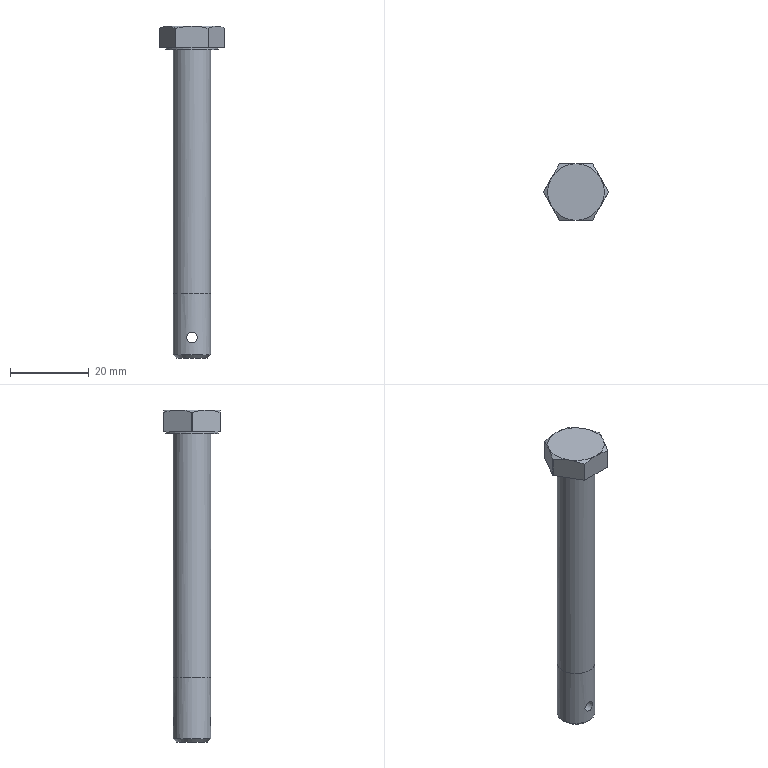Part | NX | features solid 2 | 1 solid | 27 faces | box 16.51 x 14.351 x 84.153 mm | volume 6554 mm3 | cylinder 10 | plane 10 | cone 7 | commonest cylinder face diameters 16.51 x6 9.525 x2 2.692 x1 13.284 x1
STEP:
#1=CARTESIAN_POINT('',(0.,-4.763,-80.34));
#2=VERTEX_POINT('',#1);
#3=CARTESIAN_POINT('',(1.056,-4.667,-80.048));
#4=CARTESIAN_POINT('',(-0.0001384,-4.81,-80.486));
#5=CARTESIAN_POINT('',(-1.055,-4.667,-80.048));
#6=CARTESIAN_POINT('',(-1.492,-4.519,-78.996));
#7=CARTESIAN_POINT('',(-1.055,-4.667,-77.939));
#8=CARTESIAN_POINT('',(-0.0007508,-4.81,-77.502));
#9=CARTESIAN_POINT('',(1.054,-4.668,-77.938));
#10=CARTESIAN_POINT('',(1.492,-4.519,-78.994));
#11=CARTESIAN_POINT('',(1.056,-4.667,-80.048));
#12=CARTESIAN_POINT('',(-0.0001384,-4.81,-80.486));
#13=CARTESIAN_POINT('',(-1.055,-4.667,-80.048));
#14=B_SPLINE_CURVE_WITH_KNOTS('',3,(#3,#4,#5,#6,#7,#8,#9,#10,#11,#12,#13),.UNSPECIFIED.,.T.,.F.,(1,1,1,1,1,1,1,1,1,1,1,1,1,1,1),(-0.003172,-0.002115,-0.001057,0.,0.001057,0.002115,0.003172,0.00423,0.005287,0.006345,0.007402,0.00846,0.009517,0.01057,0.01163),.UNSPECIFIED.);
#15=EDGE_CURVE('',#2,#2,#14,.T.);
#16=ORIENTED_EDGE('',*,*,#15,.T.);
#17=EDGE_LOOP('',(#16));
#18=FACE_BOUND('',#17,.T.);
#19=CARTESIAN_POINT('',(-4.763,0.,-67.882));
#20=VERTEX_POINT('',#19);
#21=CARTESIAN_POINT('',(-3.732,3.732,-67.882));
#22=CARTESIAN_POINT('',(-5.278,0.,-67.882));
#23=CARTESIAN_POINT('',(-3.732,-3.732,-67.882));
#24=CARTESIAN_POINT('',(0.,-5.278,-67.882));
#25=CARTESIAN_POINT('',(3.732,-3.732,-67.882));
#26=CARTESIAN_POINT('',(5.278,0.,-67.882));
#27=CARTESIAN_POINT('',(3.732,3.732,-67.882));
#28=CARTESIAN_POINT('',(0.,5.278,-67.882));
#29=CARTESIAN_POINT('',(-3.732,3.732,-67.882));
#30=CARTESIAN_POINT('',(-5.278,0.,-67.882));
#31=CARTESIAN_POINT('',(-3.732,-3.732,-67.882));
#32=B_SPLINE_CURVE_WITH_KNOTS('',3,(#21,#22,#23,#24,#25,#26,#27,#28,#29,#30,#31),.UNSPECIFIED.,.T.,.F.,(1,1,1,1,1,1,1,1,1,1,1,1,1,1,1),(-0.375,-0.25,-0.125,0.,0.125,0.25,0.375,0.5,0.625,0.75,0.875,1.,1.125,1.25,1.375),.UNSPECIFIED.);
#33=EDGE_CURVE('',#20,#20,#32,.T.);
#34=ORIENTED_EDGE('',*,*,#33,.F.);
#35=EDGE_LOOP('',(#34));
#36=FACE_BOUND('',#35,.T.);
#37=CARTESIAN_POINT('',(-4.763,0.,-83.366));
#38=VERTEX_POINT('',#37);
#39=CARTESIAN_POINT('',(0.,0.,-83.366));
#40=DIRECTION('',(0.,0.,-1.));
#41=DIRECTION('',(-1.,0.,0.));
#42=AXIS2_PLACEMENT_3D('',#39,#40,#41);
#43=CIRCLE('',#42,4.763);
#44=EDGE_CURVE('',#38,#38,#43,.T.);
#45=ORIENTED_EDGE('',*,*,#44,.F.);
#46=EDGE_LOOP('',(#45));
#47=FACE_BOUND('',#46,.T.);
#48=CARTESIAN_POINT('',(0.,4.763,-80.34));
#49=VERTEX_POINT('',#48);
#50=CARTESIAN_POINT('',(-1.056,4.667,-80.048));
#51=CARTESIAN_POINT('',(0.0001384,4.81,-80.486));
#52=CARTESIAN_POINT('',(1.055,4.667,-80.048));
#53=CARTESIAN_POINT('',(1.492,4.519,-78.996));
#54=CARTESIAN_POINT('',(1.055,4.667,-77.939));
#55=CARTESIAN_POINT('',(0.0007508,4.81,-77.502));
#56=CARTESIAN_POINT('',(-1.054,4.668,-77.938));
#57=CARTESIAN_POINT('',(-1.492,4.519,-78.994));
#58=CARTESIAN_POINT('',(-1.056,4.667,-80.048));
#59=CARTESIAN_POINT('',(0.0001384,4.81,-80.486));
#60=CARTESIAN_POINT('',(1.055,4.667,-80.048));
#61=B_SPLINE_CURVE_WITH_KNOTS('',3,(#50,#51,#52,#53,#54,#55,#56,#57,#58,#59,#60),.UNSPECIFIED.,.T.,.F.,(1,1,1,1,1,1,1,1,1,1,1,1,1,1,1),(-0.003172,-0.002115,-0.001057,0.,0.001057,0.002115,0.003172,0.00423,0.005287,0.006345,0.007402,0.00846,0.009517,0.01057,0.01163),.UNSPECIFIED.);
#62=EDGE_CURVE('',#49,#49,#61,.T.);
#63=ORIENTED_EDGE('',*,*,#62,.T.);
#64=EDGE_LOOP('',(#63));
#65=FACE_BOUND('',#64,.T.);
#66=CARTESIAN_POINT('',(0.,0.,0.));
#67=DIRECTION('',(0.,0.,-1.));
#68=DIRECTION('',(-1.,0.,0.));
#69=AXIS2_PLACEMENT_3D('',#66,#67,#68);
#70=CYLINDRICAL_SURFACE('',#69,4.763);
#71=ADVANCED_FACE('',(#18,#36,#47,#65),#70,.T.);
#72=CARTESIAN_POINT('',(-4.763,0.,-5.969));
#73=VERTEX_POINT('',#72);
#74=CARTESIAN_POINT('',(0.,0.,-5.969));
#75=DIRECTION('',(0.,0.,-1.));
#76=DIRECTION('',(-1.,0.,0.));
#77=AXIS2_PLACEMENT_3D('',#74,#75,#76);
#78=CIRCLE('',#77,4.763);
#79=EDGE_CURVE('',#73,#73,#78,.T.);
#80=ORIENTED_EDGE('',*,*,#79,.T.);
#81=EDGE_LOOP('',(#80));
#82=FACE_BOUND('',#81,.T.);
#83=ORIENTED_EDGE('',*,*,#33,.T.);
#84=EDGE_LOOP('',(#83));
#85=FACE_BOUND('',#84,.T.);
#86=CARTESIAN_POINT('',(0.,0.,0.));
#87=DIRECTION('',(0.,0.,-1.));
#88=DIRECTION('',(-1.,0.,0.));
#89=AXIS2_PLACEMENT_3D('',#86,#87,#88);
#90=CYLINDRICAL_SURFACE('',#89,4.763);
#91=ADVANCED_FACE('',(#82,#85),#90,.T.);
#92=CARTESIAN_POINT('',(4.081,7.176,-5.563));
#93=VERTEX_POINT('',#92);
#94=CARTESIAN_POINT('',(4.174,7.122,-5.563));
#95=VERTEX_POINT('',#94);
#96=CARTESIAN_POINT('',(0.,0.,-5.563));
#97=DIRECTION('',(0.,0.,-1.));
#98=DIRECTION('',(-1.,0.,0.));
#99=AXIS2_PLACEMENT_3D('',#96,#97,#98);
#100=CIRCLE('',#99,8.255);
#101=EDGE_CURVE('',#93,#95,#100,.T.);
#102=ORIENTED_EDGE('',*,*,#101,.F.);
#103=CARTESIAN_POINT('',(4.081,7.176,-0.6232));
#104=VERTEX_POINT('',#103);
#105=CARTESIAN_POINT('',(4.081,7.176,0.));
#106=DIRECTION('',(0.,0.,-1.));
#107=VECTOR('',#106,1000.);
#108=LINE('',#105,#107);
#109=EDGE_CURVE('',#93,#104,#108,.F.);
#110=ORIENTED_EDGE('',*,*,#109,.T.);
#111=CARTESIAN_POINT('',(4.174,7.122,-0.6232));
#112=VERTEX_POINT('',#111);
#113=CARTESIAN_POINT('',(0.,0.,-0.6232));
#114=DIRECTION('',(0.,0.,-1.));
#115=DIRECTION('',(-1.,0.,0.));
#116=AXIS2_PLACEMENT_3D('',#113,#114,#115);
#117=CIRCLE('',#116,8.255);
#118=EDGE_CURVE('',#104,#112,#117,.T.);
#119=ORIENTED_EDGE('',*,*,#118,.T.);
#120=CARTESIAN_POINT('',(4.174,7.122,0.));
#121=DIRECTION('',(0.,0.,-1.));
#122=VECTOR('',#121,1000.);
#123=LINE('',#120,#122);
#124=EDGE_CURVE('',#112,#95,#123,.T.);
#125=ORIENTED_EDGE('',*,*,#124,.T.);
#126=EDGE_LOOP('',(#102,#110,#119,#125));
#127=FACE_BOUND('',#126,.T.);
#128=CARTESIAN_POINT('',(0.,0.,0.));
#129=DIRECTION('',(0.,0.,-1.));
#130=DIRECTION('',(-1.,0.,0.));
#131=AXIS2_PLACEMENT_3D('',#128,#129,#130);
#132=CYLINDRICAL_SURFACE('',#131,8.255);
#133=ADVANCED_FACE('',(#127),#132,.T.);
#134=CARTESIAN_POINT('',(-4.174,7.122,-0.6232));
#135=VERTEX_POINT('',#134);
#136=CARTESIAN_POINT('',(-4.081,7.176,-0.6232));
#137=VERTEX_POINT('',#136);
#138=CARTESIAN_POINT('',(0.,0.,-0.6232));
#139=DIRECTION('',(0.,0.,-1.));
#140=DIRECTION('',(-1.,0.,0.));
#141=AXIS2_PLACEMENT_3D('',#138,#139,#140);
#142=CIRCLE('',#141,8.255);
#143=EDGE_CURVE('',#135,#137,#142,.T.);
#144=ORIENTED_EDGE('',*,*,#143,.T.);
#145=CARTESIAN_POINT('',(-4.081,7.176,-5.563));
#146=VERTEX_POINT('',#145);
#147=CARTESIAN_POINT('',(-4.081,7.176,0.));
#148=DIRECTION('',(0.,0.,-1.));
#149=VECTOR('',#148,1000.);
#150=LINE('',#147,#149);
#151=EDGE_CURVE('',#137,#146,#150,.T.);
#152=ORIENTED_EDGE('',*,*,#151,.T.);
#153=CARTESIAN_POINT('',(-4.174,7.122,-5.563));
#154=VERTEX_POINT('',#153);
#155=CARTESIAN_POINT('',(0.,0.,-5.563));
#156=DIRECTION('',(0.,0.,-1.));
#157=DIRECTION('',(-1.,0.,0.));
#158=AXIS2_PLACEMENT_3D('',#155,#156,#157);
#159=CIRCLE('',#158,8.255);
#160=EDGE_CURVE('',#154,#146,#159,.T.);
#161=ORIENTED_EDGE('',*,*,#160,.F.);
#162=CARTESIAN_POINT('',(-4.174,7.122,0.));
#163=DIRECTION('',(0.,0.,-1.));
#164=VECTOR('',#163,1000.);
#165=LINE('',#162,#164);
#166=EDGE_CURVE('',#154,#135,#165,.F.);
#167=ORIENTED_EDGE('',*,*,#166,.T.);
#168=EDGE_LOOP('',(#144,#152,#161,#167));
#169=FACE_BOUND('',#168,.T.);
#170=CARTESIAN_POINT('',(0.,0.,0.));
#171=DIRECTION('',(0.,0.,-1.));
#172=DIRECTION('',(-1.,0.,0.));
#173=AXIS2_PLACEMENT_3D('',#170,#171,#172);
#174=CYLINDRICAL_SURFACE('',#173,8.255);
#175=ADVANCED_FACE('',(#169),#174,.T.);
#176=CARTESIAN_POINT('',(-8.255,-0.05322,-0.6232));
#177=VERTEX_POINT('',#176);
#178=CARTESIAN_POINT('',(-8.255,0.05322,-0.6232));
#179=VERTEX_POINT('',#178);
#180=CARTESIAN_POINT('',(0.,0.,-0.6232));
#181=DIRECTION('',(0.,0.,-1.));
#182=DIRECTION('',(-1.,0.,0.));
#183=AXIS2_PLACEMENT_3D('',#180,#181,#182);
#184=CIRCLE('',#183,8.255);
#185=EDGE_CURVE('',#177,#179,#184,.T.);
#186=ORIENTED_EDGE('',*,*,#185,.T.);
#187=CARTESIAN_POINT('',(-8.255,0.05322,-5.563));
#188=VERTEX_POINT('',#187);
#189=CARTESIAN_POINT('',(-8.255,0.05322,0.));
#190=DIRECTION('',(0.,0.,-1.));
#191=VECTOR('',#190,1000.);
#192=LINE('',#189,#191);
#193=EDGE_CURVE('',#179,#188,#192,.T.);
#194=ORIENTED_EDGE('',*,*,#193,.T.);
#195=CARTESIAN_POINT('',(-8.255,-0.05322,-5.563));
#196=VERTEX_POINT('',#195);
#197=CARTESIAN_POINT('',(0.,0.,-5.563));
#198=DIRECTION('',(0.,0.,-1.));
#199=DIRECTION('',(-1.,0.,0.));
#200=AXIS2_PLACEMENT_3D('',#197,#198,#199);
#201=CIRCLE('',#200,8.255);
#202=EDGE_CURVE('',#196,#188,#201,.T.);
#203=ORIENTED_EDGE('',*,*,#202,.F.);
#204=CARTESIAN_POINT('',(-8.255,-0.05322,0.));
#205=DIRECTION('',(0.,0.,-1.));
#206=VECTOR('',#205,1000.);
#207=LINE('',#204,#206);
#208=EDGE_CURVE('',#196,#177,#207,.F.);
#209=ORIENTED_EDGE('',*,*,#208,.T.);
#210=EDGE_LOOP('',(#186,#194,#203,#209));
#211=FACE_BOUND('',#210,.T.);
#212=CARTESIAN_POINT('',(0.,0.,0.));
#213=DIRECTION('',(0.,0.,-1.));
#214=DIRECTION('',(-1.,0.,0.));
#215=AXIS2_PLACEMENT_3D('',#212,#213,#214);
#216=CYLINDRICAL_SURFACE('',#215,8.255);
#217=ADVANCED_FACE('',(#211),#216,.T.);
#218=CARTESIAN_POINT('',(-4.081,-7.176,-0.6232));
#219=VERTEX_POINT('',#218);
#220=CARTESIAN_POINT('',(-4.174,-7.122,-0.6232));
#221=VERTEX_POINT('',#220);
#222=CARTESIAN_POINT('',(0.,0.,-0.6232));
#223=DIRECTION('',(0.,0.,-1.));
#224=DIRECTION('',(-1.,0.,0.));
#225=AXIS2_PLACEMENT_3D('',#222,#223,#224);
#226=CIRCLE('',#225,8.255);
#227=EDGE_CURVE('',#219,#221,#226,.T.);
#228=ORIENTED_EDGE('',*,*,#227,.T.);
#229=CARTESIAN_POINT('',(-4.174,-7.122,-5.563));
#230=VERTEX_POINT('',#229);
#231=CARTESIAN_POINT('',(-4.174,-7.122,0.));
#232=DIRECTION('',(0.,0.,-1.));
#233=VECTOR('',#232,1000.);
#234=LINE('',#231,#233);
#235=EDGE_CURVE('',#221,#230,#234,.T.);
#236=ORIENTED_EDGE('',*,*,#235,.T.);
#237=CARTESIAN_POINT('',(-4.081,-7.176,-5.563));
#238=VERTEX_POINT('',#237);
#239=CARTESIAN_POINT('',(0.,0.,-5.563));
#240=DIRECTION('',(0.,0.,-1.));
#241=DIRECTION('',(-1.,0.,0.));
#242=AXIS2_PLACEMENT_3D('',#239,#240,#241);
#243=CIRCLE('',#242,8.255);
#244=EDGE_CURVE('',#238,#230,#243,.T.);
#245=ORIENTED_EDGE('',*,*,#244,.F.);
#246=CARTESIAN_POINT('',(-4.081,-7.176,0.));
#247=DIRECTION('',(0.,0.,-1.));
#248=VECTOR('',#247,1000.);
#249=LINE('',#246,#248);
#250=EDGE_CURVE('',#238,#219,#249,.F.);
#251=ORIENTED_EDGE('',*,*,#250,.T.);
#252=EDGE_LOOP('',(#228,#236,#245,#251));
#253=FACE_BOUND('',#252,.T.);
#254=CARTESIAN_POINT('',(0.,0.,0.));
#255=DIRECTION('',(0.,0.,-1.));
#256=DIRECTION('',(-1.,0.,0.));
#257=AXIS2_PLACEMENT_3D('',#254,#255,#256);
#258=CYLINDRICAL_SURFACE('',#257,8.255);
#259=ADVANCED_FACE('',(#253),#258,.T.);
#260=CARTESIAN_POINT('',(4.174,-7.122,-0.6232));
#261=VERTEX_POINT('',#260);
#262=CARTESIAN_POINT('',(4.081,-7.176,-0.6232));
#263=VERTEX_POINT('',#262);
#264=CARTESIAN_POINT('',(0.,0.,-0.6232));
#265=DIRECTION('',(0.,0.,-1.));
#266=DIRECTION('',(-1.,0.,0.));
#267=AXIS2_PLACEMENT_3D('',#264,#265,#266);
#268=CIRCLE('',#267,8.255);
#269=EDGE_CURVE('',#261,#263,#268,.T.);
#270=ORIENTED_EDGE('',*,*,#269,.T.);
#271=CARTESIAN_POINT('',(4.081,-7.176,-5.563));
#272=VERTEX_POINT('',#271);
#273=CARTESIAN_POINT('',(4.081,-7.176,0.));
#274=DIRECTION('',(0.,0.,-1.));
#275=VECTOR('',#274,1000.);
#276=LINE('',#273,#275);
#277=EDGE_CURVE('',#263,#272,#276,.T.);
#278=ORIENTED_EDGE('',*,*,#277,.T.);
#279=CARTESIAN_POINT('',(4.174,-7.122,-5.563));
#280=VERTEX_POINT('',#279);
#281=CARTESIAN_POINT('',(0.,0.,-5.563));
#282=DIRECTION('',(0.,0.,-1.));
#283=DIRECTION('',(-1.,0.,0.));
#284=AXIS2_PLACEMENT_3D('',#281,#282,#283);
#285=CIRCLE('',#284,8.255);
#286=EDGE_CURVE('',#280,#272,#285,.T.);
#287=ORIENTED_EDGE('',*,*,#286,.F.);
#288=CARTESIAN_POINT('',(4.174,-7.122,0.));
#289=DIRECTION('',(0.,0.,-1.));
#290=VECTOR('',#289,1000.);
#291=LINE('',#288,#290);
#292=EDGE_CURVE('',#280,#261,#291,.F.);
#293=ORIENTED_EDGE('',*,*,#292,.T.);
#294=EDGE_LOOP('',(#270,#278,#287,#293));
#295=FACE_BOUND('',#294,.T.);
#296=CARTESIAN_POINT('',(0.,0.,0.));
#297=DIRECTION('',(0.,0.,-1.));
#298=DIRECTION('',(-1.,0.,0.));
#299=AXIS2_PLACEMENT_3D('',#296,#297,#298);
#300=CYLINDRICAL_SURFACE('',#299,8.255);
#301=ADVANCED_FACE('',(#295),#300,.T.);
#302=ORIENTED_EDGE('',*,*,#118,.F.);
#303=CARTESIAN_POINT('',(0.,7.176,0.));
#304=VERTEX_POINT('',#303);
#305=CARTESIAN_POINT('',(0.,7.176,0.));
#306=CARTESIAN_POINT('',(1.38,7.176,0.));
#307=CARTESIAN_POINT('',(2.761,7.176,-0.2464));
#308=CARTESIAN_POINT('',(4.081,7.176,-0.6232));
#309=B_SPLINE_CURVE_WITH_KNOTS('',3,(#305,#306,#307,#308),.UNSPECIFIED.,.F.,.F.,(4,4),(0.01158,0.01571),.UNSPECIFIED.);
#310=EDGE_CURVE('',#104,#304,#309,.F.);
#311=ORIENTED_EDGE('',*,*,#310,.T.);
#312=CARTESIAN_POINT('',(6.214,3.588,0.));
#313=VERTEX_POINT('',#312);
#314=CARTESIAN_POINT('',(0.,0.,0.));
#315=DIRECTION('',(0.,0.,-1.));
#316=DIRECTION('',(-1.,0.,0.));
#317=AXIS2_PLACEMENT_3D('',#314,#315,#316);
#318=CIRCLE('',#317,7.176);
#319=EDGE_CURVE('',#304,#313,#318,.T.);
#320=ORIENTED_EDGE('',*,*,#319,.T.);
#321=CARTESIAN_POINT('',(6.214,3.588,0.));
#322=CARTESIAN_POINT('',(5.522,4.786,0.));
#323=CARTESIAN_POINT('',(4.84,5.968,-0.2429));
#324=CARTESIAN_POINT('',(4.174,7.122,-0.6232));
#325=B_SPLINE_CURVE_WITH_KNOTS('',3,(#321,#322,#323,#324),.UNSPECIFIED.,.F.,.F.,(4,4),(0.004129,0.00824),.UNSPECIFIED.);
#326=EDGE_CURVE('',#313,#112,#325,.T.);
#327=ORIENTED_EDGE('',*,*,#326,.T.);
#328=EDGE_LOOP('',(#302,#311,#320,#327));
#329=FACE_BOUND('',#328,.T.);
#330=CARTESIAN_POINT('',(0.,0.,-0.6232));
#331=DIRECTION('',(0.,0.,-1.));
#332=DIRECTION('',(-1.,0.,0.));
#333=AXIS2_PLACEMENT_3D('',#330,#331,#332);
#334=CONICAL_SURFACE('',#333,8.255,1.047);
#335=ADVANCED_FACE('',(#329),#334,.T.);
#336=CARTESIAN_POINT('',(-6.214,3.588,0.));
#337=VERTEX_POINT('',#336);
#338=CARTESIAN_POINT('',(0.,0.,0.));
#339=DIRECTION('',(0.,0.,-1.));
#340=DIRECTION('',(-1.,0.,0.));
#341=AXIS2_PLACEMENT_3D('',#338,#339,#340);
#342=CIRCLE('',#341,7.176);
#343=EDGE_CURVE('',#337,#304,#342,.T.);
#344=ORIENTED_EDGE('',*,*,#343,.T.);
#345=CARTESIAN_POINT('',(-4.081,7.176,-0.6232));
#346=CARTESIAN_POINT('',(-2.753,7.176,-0.244));
#347=CARTESIAN_POINT('',(-1.379,7.176,0.));
#348=CARTESIAN_POINT('',(0.,7.176,0.));
#349=B_SPLINE_CURVE_WITH_KNOTS('',3,(#345,#346,#347,#348),.UNSPECIFIED.,.F.,.F.,(4,4),(0.007452,0.01158),.UNSPECIFIED.);
#350=EDGE_CURVE('',#304,#137,#349,.F.);
#351=ORIENTED_EDGE('',*,*,#350,.T.);
#352=ORIENTED_EDGE('',*,*,#143,.F.);
#353=CARTESIAN_POINT('',(-4.174,7.122,-0.6232));
#354=CARTESIAN_POINT('',(-4.842,5.965,-0.2418));
#355=CARTESIAN_POINT('',(-5.519,4.791,0.));
#356=CARTESIAN_POINT('',(-6.214,3.588,0.));
#357=B_SPLINE_CURVE_WITH_KNOTS('',3,(#353,#354,#355,#356),.UNSPECIFIED.,.F.,.F.,(4,4),(0.000000722,0.004129),.UNSPECIFIED.);
#358=EDGE_CURVE('',#135,#337,#357,.T.);
#359=ORIENTED_EDGE('',*,*,#358,.T.);
#360=EDGE_LOOP('',(#344,#351,#352,#359));
#361=FACE_BOUND('',#360,.T.);
#362=CARTESIAN_POINT('',(0.,0.,-0.6232));
#363=DIRECTION('',(0.,0.,-1.));
#364=DIRECTION('',(-1.,0.,0.));
#365=AXIS2_PLACEMENT_3D('',#362,#363,#364);
#366=CONICAL_SURFACE('',#365,8.255,1.047);
#367=ADVANCED_FACE('',(#361),#366,.T.);
#368=CARTESIAN_POINT('',(-6.214,-3.588,0.));
#369=VERTEX_POINT('',#368);
#370=CARTESIAN_POINT('',(0.,0.,0.));
#371=DIRECTION('',(0.,0.,-1.));
#372=DIRECTION('',(-1.,0.,0.));
#373=AXIS2_PLACEMENT_3D('',#370,#371,#372);
#374=CIRCLE('',#373,7.176);
#375=EDGE_CURVE('',#369,#337,#374,.T.);
#376=ORIENTED_EDGE('',*,*,#375,.T.);
#377=CARTESIAN_POINT('',(-6.214,3.588,0.));
#378=CARTESIAN_POINT('',(-6.906,2.389,0.));
#379=CARTESIAN_POINT('',(-7.589,1.207,-0.2429));
#380=CARTESIAN_POINT('',(-8.255,0.05322,-0.6232));
#381=B_SPLINE_CURVE_WITH_KNOTS('',3,(#377,#378,#379,#380),.UNSPECIFIED.,.F.,.F.,(4,4),(0.004129,0.00824),.UNSPECIFIED.);
#382=EDGE_CURVE('',#337,#179,#381,.T.);
#383=ORIENTED_EDGE('',*,*,#382,.T.);
#384=ORIENTED_EDGE('',*,*,#185,.F.);
#385=CARTESIAN_POINT('',(-8.255,-0.05322,-0.6232));
#386=CARTESIAN_POINT('',(-7.587,-1.21,-0.2418));
#387=CARTESIAN_POINT('',(-6.909,-2.384,0.));
#388=CARTESIAN_POINT('',(-6.214,-3.588,0.));
#389=B_SPLINE_CURVE_WITH_KNOTS('',3,(#385,#386,#387,#388),.UNSPECIFIED.,.F.,.F.,(4,4),(0.000000722,0.004129),.UNSPECIFIED.);
#390=EDGE_CURVE('',#177,#369,#389,.T.);
#391=ORIENTED_EDGE('',*,*,#390,.T.);
#392=EDGE_LOOP('',(#376,#383,#384,#391));
#393=FACE_BOUND('',#392,.T.);
#394=CARTESIAN_POINT('',(0.,0.,-0.6232));
#395=DIRECTION('',(0.,0.,-1.));
#396=DIRECTION('',(-1.,0.,0.));
#397=AXIS2_PLACEMENT_3D('',#394,#395,#396);
#398=CONICAL_SURFACE('',#397,8.255,1.047);
#399=ADVANCED_FACE('',(#393),#398,.T.);
#400=CARTESIAN_POINT('',(0.,-7.176,0.));
#401=VERTEX_POINT('',#400);
#402=CARTESIAN_POINT('',(0.,0.,0.));
#403=DIRECTION('',(0.,0.,-1.));
#404=DIRECTION('',(-1.,0.,0.));
#405=AXIS2_PLACEMENT_3D('',#402,#403,#404);
#406=CIRCLE('',#405,7.176);
#407=EDGE_CURVE('',#401,#369,#406,.T.);
#408=ORIENTED_EDGE('',*,*,#407,.T.);
#409=CARTESIAN_POINT('',(-6.214,-3.588,0.));
#410=CARTESIAN_POINT('',(-5.522,-4.786,0.));
#411=CARTESIAN_POINT('',(-4.84,-5.968,-0.2429));
#412=CARTESIAN_POINT('',(-4.174,-7.122,-0.6232));
#413=B_SPLINE_CURVE_WITH_KNOTS('',3,(#409,#410,#411,#412),.UNSPECIFIED.,.F.,.F.,(4,4),(0.004129,0.00824),.UNSPECIFIED.);
#414=EDGE_CURVE('',#369,#221,#413,.T.);
#415=ORIENTED_EDGE('',*,*,#414,.T.);
#416=ORIENTED_EDGE('',*,*,#227,.F.);
#417=CARTESIAN_POINT('',(-4.081,-7.176,-0.6232));
#418=CARTESIAN_POINT('',(-2.753,-7.176,-0.244));
#419=CARTESIAN_POINT('',(-1.379,-7.176,0.));
#420=CARTESIAN_POINT('',(0.,-7.176,0.));
#421=B_SPLINE_CURVE_WITH_KNOTS('',3,(#417,#418,#419,#420),.UNSPECIFIED.,.F.,.F.,(4,4),(0.007452,0.01158),.UNSPECIFIED.);
#422=EDGE_CURVE('',#219,#401,#421,.T.);
#423=ORIENTED_EDGE('',*,*,#422,.T.);
#424=EDGE_LOOP('',(#408,#415,#416,#423));
#425=FACE_BOUND('',#424,.T.);
#426=CARTESIAN_POINT('',(0.,0.,-0.6232));
#427=DIRECTION('',(0.,0.,-1.));
#428=DIRECTION('',(-1.,0.,0.));
#429=AXIS2_PLACEMENT_3D('',#426,#427,#428);
#430=CONICAL_SURFACE('',#429,8.255,1.047);
#431=ADVANCED_FACE('',(#425),#430,.T.);
#432=CARTESIAN_POINT('',(6.214,-3.588,0.));
#433=VERTEX_POINT('',#432);
#434=CARTESIAN_POINT('',(0.,0.,0.));
#435=DIRECTION('',(0.,0.,-1.));
#436=DIRECTION('',(-1.,0.,0.));
#437=AXIS2_PLACEMENT_3D('',#434,#435,#436);
#438=CIRCLE('',#437,7.176);
#439=EDGE_CURVE('',#433,#401,#438,.T.);
#440=ORIENTED_EDGE('',*,*,#439,.T.);
#441=CARTESIAN_POINT('',(0.,-7.176,0.));
#442=CARTESIAN_POINT('',(1.38,-7.176,0.));
#443=CARTESIAN_POINT('',(2.761,-7.176,-0.2464));
#444=CARTESIAN_POINT('',(4.081,-7.176,-0.6232));
#445=B_SPLINE_CURVE_WITH_KNOTS('',3,(#441,#442,#443,#444),.UNSPECIFIED.,.F.,.F.,(4,4),(0.01158,0.01571),.UNSPECIFIED.);
#446=EDGE_CURVE('',#401,#263,#445,.T.);
#447=ORIENTED_EDGE('',*,*,#446,.T.);
#448=ORIENTED_EDGE('',*,*,#269,.F.);
#449=CARTESIAN_POINT('',(4.174,-7.122,-0.6232));
#450=CARTESIAN_POINT('',(4.842,-5.965,-0.2418));
#451=CARTESIAN_POINT('',(5.519,-4.791,0.));
#452=CARTESIAN_POINT('',(6.214,-3.588,0.));
#453=B_SPLINE_CURVE_WITH_KNOTS('',3,(#449,#450,#451,#452),.UNSPECIFIED.,.F.,.F.,(4,4),(0.000000722,0.004129),.UNSPECIFIED.);
#454=EDGE_CURVE('',#261,#433,#453,.T.);
#455=ORIENTED_EDGE('',*,*,#454,.T.);
#456=EDGE_LOOP('',(#440,#447,#448,#455));
#457=FACE_BOUND('',#456,.T.);
#458=CARTESIAN_POINT('',(0.,0.,-0.6232));
#459=DIRECTION('',(0.,0.,-1.));
#460=DIRECTION('',(-1.,0.,0.));
#461=AXIS2_PLACEMENT_3D('',#458,#459,#460);
#462=CONICAL_SURFACE('',#461,8.255,1.047);
#463=ADVANCED_FACE('',(#457),#462,.T.);
#464=ORIENTED_EDGE('',*,*,#160,.T.);
#465=CARTESIAN_POINT('',(6.642,7.176,-5.563));
#466=DIRECTION('',(1.,0.,0.));
#467=VECTOR('',#466,1000.);
#468=LINE('',#465,#467);
#469=EDGE_CURVE('',#146,#93,#468,.T.);
#470=ORIENTED_EDGE('',*,*,#469,.T.);
#471=ORIENTED_EDGE('',*,*,#101,.T.);
#472=CARTESIAN_POINT('',(8.255,0.05322,-5.563));
#473=VERTEX_POINT('',#472);
#474=CARTESIAN_POINT('',(7.875,0.7116,-5.563));
#475=DIRECTION('',(0.5,-0.866,0.));
#476=VECTOR('',#475,1000.);
#477=LINE('',#474,#476);
#478=EDGE_CURVE('',#95,#473,#477,.T.);
#479=ORIENTED_EDGE('',*,*,#478,.T.);
#480=CARTESIAN_POINT('',(8.255,-0.05322,-5.563));
#481=VERTEX_POINT('',#480);
#482=CARTESIAN_POINT('',(0.,0.,-5.563));
#483=DIRECTION('',(0.,0.,-1.));
#484=DIRECTION('',(-1.,0.,0.));
#485=AXIS2_PLACEMENT_3D('',#482,#483,#484);
#486=CIRCLE('',#485,8.255);
#487=EDGE_CURVE('',#473,#481,#486,.T.);
#488=ORIENTED_EDGE('',*,*,#487,.T.);
#489=CARTESIAN_POINT('',(7.875,-0.7116,-5.563));
#490=DIRECTION('',(-0.5,-0.866,0.));
#491=VECTOR('',#490,1000.);
#492=LINE('',#489,#491);
#493=EDGE_CURVE('',#481,#280,#492,.T.);
#494=ORIENTED_EDGE('',*,*,#493,.T.);
#495=ORIENTED_EDGE('',*,*,#286,.T.);
#496=CARTESIAN_POINT('',(6.642,-7.176,-5.563));
#497=DIRECTION('',(-1.,0.,0.));
#498=VECTOR('',#497,1000.);
#499=LINE('',#496,#498);
#500=EDGE_CURVE('',#272,#238,#499,.T.);
#501=ORIENTED_EDGE('',*,*,#500,.T.);
#502=ORIENTED_EDGE('',*,*,#244,.T.);
#503=CARTESIAN_POINT('',(-4.554,-6.464,-5.563));
#504=DIRECTION('',(-0.5,0.866,0.));
#505=VECTOR('',#504,1000.);
#506=LINE('',#503,#505);
#507=EDGE_CURVE('',#230,#196,#506,.T.);
#508=ORIENTED_EDGE('',*,*,#507,.T.);
#509=ORIENTED_EDGE('',*,*,#202,.T.);
#510=CARTESIAN_POINT('',(-4.554,6.464,-5.563));
#511=DIRECTION('',(0.5,0.866,0.));
#512=VECTOR('',#511,1000.);
#513=LINE('',#510,#512);
#514=EDGE_CURVE('',#188,#154,#513,.T.);
#515=ORIENTED_EDGE('',*,*,#514,.T.);
#516=EDGE_LOOP('',(#464,#470,#471,#479,#488,#494,#495,#501,#502,#508,#509,#515));
#517=FACE_BOUND('',#516,.T.);
#518=CARTESIAN_POINT('',(-6.642,0.,-5.563));
#519=VERTEX_POINT('',#518);
#520=CARTESIAN_POINT('',(0.,0.,-5.563));
#521=DIRECTION('',(0.,0.,-1.));
#522=DIRECTION('',(-1.,0.,0.));
#523=AXIS2_PLACEMENT_3D('',#520,#521,#522);
#524=CIRCLE('',#523,6.642);
#525=EDGE_CURVE('',#519,#519,#524,.T.);
#526=ORIENTED_EDGE('',*,*,#525,.F.);
#527=EDGE_LOOP('',(#526));
#528=FACE_BOUND('',#527,.T.);
#529=CARTESIAN_POINT('',(6.642,0.,-5.563));
#530=DIRECTION('',(0.,0.,-1.));
#531=DIRECTION('',(-1.,0.,0.));
#532=AXIS2_PLACEMENT_3D('',#529,#530,#531);
#533=PLANE('',#532);
#534=ADVANCED_FACE('',(#517,#528),#533,.T.);
#535=CARTESIAN_POINT('',(8.255,0.05322,-0.6232));
#536=VERTEX_POINT('',#535);
#537=CARTESIAN_POINT('',(8.255,-0.05322,-0.6232));
#538=VERTEX_POINT('',#537);
#539=CARTESIAN_POINT('',(0.,0.,-0.6232));
#540=DIRECTION('',(0.,0.,-1.));
#541=DIRECTION('',(-1.,0.,0.));
#542=AXIS2_PLACEMENT_3D('',#539,#540,#541);
#543=CIRCLE('',#542,8.255);
#544=EDGE_CURVE('',#536,#538,#543,.T.);
#545=ORIENTED_EDGE('',*,*,#544,.T.);
#546=CARTESIAN_POINT('',(8.255,-0.05322,0.));
#547=DIRECTION('',(0.,0.,-1.));
#548=VECTOR('',#547,1000.);
#549=LINE('',#546,#548);
#550=EDGE_CURVE('',#538,#481,#549,.T.);
#551=ORIENTED_EDGE('',*,*,#550,.T.);
#552=ORIENTED_EDGE('',*,*,#487,.F.);
#553=CARTESIAN_POINT('',(8.255,0.05322,0.));
#554=DIRECTION('',(0.,0.,-1.));
#555=VECTOR('',#554,1000.);
#556=LINE('',#553,#555);
#557=EDGE_CURVE('',#473,#536,#556,.F.);
#558=ORIENTED_EDGE('',*,*,#557,.T.);
#559=EDGE_LOOP('',(#545,#551,#552,#558));
#560=FACE_BOUND('',#559,.T.);
#561=CARTESIAN_POINT('',(0.,0.,0.));
#562=DIRECTION('',(0.,0.,-1.));
#563=DIRECTION('',(-1.,0.,0.));
#564=AXIS2_PLACEMENT_3D('',#561,#562,#563);
#565=CYLINDRICAL_SURFACE('',#564,8.255);
#566=ADVANCED_FACE('',(#560),#565,.T.);
#567=CARTESIAN_POINT('',(0.,0.,0.));
#568=DIRECTION('',(0.,0.,-1.));
#569=DIRECTION('',(-1.,0.,0.));
#570=AXIS2_PLACEMENT_3D('',#567,#568,#569);
#571=CIRCLE('',#570,7.176);
#572=EDGE_CURVE('',#313,#433,#571,.T.);
#573=ORIENTED_EDGE('',*,*,#572,.T.);
#574=CARTESIAN_POINT('',(6.214,-3.588,0.));
#575=CARTESIAN_POINT('',(6.906,-2.389,0.));
#576=CARTESIAN_POINT('',(7.589,-1.207,-0.2429));
#577=CARTESIAN_POINT('',(8.255,-0.05322,-0.6232));
#578=B_SPLINE_CURVE_WITH_KNOTS('',3,(#574,#575,#576,#577),.UNSPECIFIED.,.F.,.F.,(4,4),(0.004129,0.00824),.UNSPECIFIED.);
#579=EDGE_CURVE('',#433,#538,#578,.T.);
#580=ORIENTED_EDGE('',*,*,#579,.T.);
#581=ORIENTED_EDGE('',*,*,#544,.F.);
#582=CARTESIAN_POINT('',(8.255,0.05322,-0.6232));
#583=CARTESIAN_POINT('',(7.587,1.21,-0.2418));
#584=CARTESIAN_POINT('',(6.909,2.384,0.));
#585=CARTESIAN_POINT('',(6.214,3.588,0.));
#586=B_SPLINE_CURVE_WITH_KNOTS('',3,(#582,#583,#584,#585),.UNSPECIFIED.,.F.,.F.,(4,4),(0.000000722,0.004129),.UNSPECIFIED.);
#587=EDGE_CURVE('',#536,#313,#586,.T.);
#588=ORIENTED_EDGE('',*,*,#587,.T.);
#589=EDGE_LOOP('',(#573,#580,#581,#588));
#590=FACE_BOUND('',#589,.T.);
#591=CARTESIAN_POINT('',(0.,0.,-0.6232));
#592=DIRECTION('',(0.,0.,-1.));
#593=DIRECTION('',(-1.,0.,0.));
#594=AXIS2_PLACEMENT_3D('',#591,#592,#593);
#595=CONICAL_SURFACE('',#594,8.255,1.047);
#596=ADVANCED_FACE('',(#590),#595,.T.);
#597=ORIENTED_EDGE('',*,*,#343,.F.);
#598=ORIENTED_EDGE('',*,*,#375,.F.);
#599=ORIENTED_EDGE('',*,*,#407,.F.);
#600=ORIENTED_EDGE('',*,*,#439,.F.);
#601=ORIENTED_EDGE('',*,*,#572,.F.);
#602=ORIENTED_EDGE('',*,*,#319,.F.);
#603=EDGE_LOOP('',(#597,#598,#599,#600,#601,#602));
#604=FACE_BOUND('',#603,.T.);
#605=CARTESIAN_POINT('',(7.176,0.,0.));
#606=DIRECTION('',(0.,0.,1.));
#607=DIRECTION('',(1.,0.,0.));
#608=AXIS2_PLACEMENT_3D('',#605,#606,#607);
#609=PLANE('',#608);
#610=ADVANCED_FACE('',(#604),#609,.T.);
#611=CARTESIAN_POINT('',(-3.975,0.,-84.153));
#612=VERTEX_POINT('',#611);
#613=CARTESIAN_POINT('',(0.,0.,-84.153));
#614=DIRECTION('',(0.,0.,-1.));
#615=DIRECTION('',(-1.,0.,0.));
#616=AXIS2_PLACEMENT_3D('',#613,#614,#615);
#617=CIRCLE('',#616,3.975);
#618=EDGE_CURVE('',#612,#612,#617,.T.);
#619=ORIENTED_EDGE('',*,*,#618,.T.);
#620=EDGE_LOOP('',(#619));
#621=FACE_BOUND('',#620,.T.);
#622=CARTESIAN_POINT('',(0.,0.,-84.153));
#623=DIRECTION('',(0.,0.,-1.));
#624=DIRECTION('',(-1.,0.,0.));
#625=AXIS2_PLACEMENT_3D('',#622,#623,#624);
#626=PLANE('',#625);
#627=ADVANCED_FACE('',(#621),#626,.T.);
#628=ORIENTED_EDGE('',*,*,#44,.T.);
#629=EDGE_LOOP('',(#628));
#630=FACE_BOUND('',#629,.T.);
#631=ORIENTED_EDGE('',*,*,#618,.F.);
#632=EDGE_LOOP('',(#631));
#633=FACE_BOUND('',#632,.T.);
#634=CARTESIAN_POINT('',(0.,0.,-84.153));
#635=DIRECTION('',(0.,0.,1.));
#636=DIRECTION('',(1.,0.,0.));
#637=AXIS2_PLACEMENT_3D('',#634,#635,#636);
#638=CONICAL_SURFACE('',#637,3.975,0.7854);
#639=ADVANCED_FACE('',(#630,#633),#638,.T.);
#640=CARTESIAN_POINT('',(-6.642,0.,-5.969));
#641=VERTEX_POINT('',#640);
#642=CARTESIAN_POINT('',(0.,0.,-5.969));
#643=DIRECTION('',(0.,0.,-1.));
#644=DIRECTION('',(-1.,0.,0.));
#645=AXIS2_PLACEMENT_3D('',#642,#643,#644);
#646=CIRCLE('',#645,6.642);
#647=EDGE_CURVE('',#641,#641,#646,.T.);
#648=ORIENTED_EDGE('',*,*,#647,.T.);
#649=EDGE_LOOP('',(#648));
#650=FACE_BOUND('',#649,.T.);
#651=ORIENTED_EDGE('',*,*,#79,.F.);
#652=EDGE_LOOP('',(#651));
#653=FACE_BOUND('',#652,.T.);
#654=CARTESIAN_POINT('',(4.763,0.,-5.969));
#655=DIRECTION('',(0.,0.,-1.));
#656=DIRECTION('',(-1.,0.,0.));
#657=AXIS2_PLACEMENT_3D('',#654,#655,#656);
#658=PLANE('',#657);
#659=ADVANCED_FACE('',(#650,#653),#658,.T.);
#660=ORIENTED_EDGE('',*,*,#525,.T.);
#661=EDGE_LOOP('',(#660));
#662=FACE_BOUND('',#661,.T.);
#663=ORIENTED_EDGE('',*,*,#647,.F.);
#664=EDGE_LOOP('',(#663));
#665=FACE_BOUND('',#664,.T.);
#666=CARTESIAN_POINT('',(0.,0.,0.));
#667=DIRECTION('',(0.,0.,-1.));
#668=DIRECTION('',(-1.,0.,0.));
#669=AXIS2_PLACEMENT_3D('',#666,#667,#668);
#670=CYLINDRICAL_SURFACE('',#669,6.642);
#671=ADVANCED_FACE('',(#662,#665),#670,.T.);
#672=ORIENTED_EDGE('',*,*,#478,.F.);
#673=ORIENTED_EDGE('',*,*,#124,.F.);
#674=ORIENTED_EDGE('',*,*,#326,.F.);
#675=ORIENTED_EDGE('',*,*,#587,.F.);
#676=ORIENTED_EDGE('',*,*,#557,.F.);
#677=EDGE_LOOP('',(#672,#673,#674,#675,#676));
#678=FACE_BOUND('',#677,.T.);
#679=CARTESIAN_POINT('',(8.286,0.,-92.569));
#680=DIRECTION('',(0.866,0.5,0.));
#681=DIRECTION('',(-0.5,0.866,0.));
#682=AXIS2_PLACEMENT_3D('',#679,#680,#681);
#683=PLANE('',#682);
#684=ADVANCED_FACE('',(#678),#683,.T.);
#685=ORIENTED_EDGE('',*,*,#493,.F.);
#686=ORIENTED_EDGE('',*,*,#550,.F.);
#687=ORIENTED_EDGE('',*,*,#579,.F.);
#688=ORIENTED_EDGE('',*,*,#454,.F.);
#689=ORIENTED_EDGE('',*,*,#292,.F.);
#690=EDGE_LOOP('',(#685,#686,#687,#688,#689));
#691=FACE_BOUND('',#690,.T.);
#692=CARTESIAN_POINT('',(4.143,-7.176,-92.569));
#693=DIRECTION('',(0.866,-0.5,0.));
#694=DIRECTION('',(0.5,0.866,0.));
#695=AXIS2_PLACEMENT_3D('',#692,#693,#694);
#696=PLANE('',#695);
#697=ADVANCED_FACE('',(#691),#696,.T.);
#698=ORIENTED_EDGE('',*,*,#500,.F.);
#699=ORIENTED_EDGE('',*,*,#277,.F.);
#700=ORIENTED_EDGE('',*,*,#446,.F.);
#701=ORIENTED_EDGE('',*,*,#422,.F.);
#702=ORIENTED_EDGE('',*,*,#250,.F.);
#703=EDGE_LOOP('',(#698,#699,#700,#701,#702));
#704=FACE_BOUND('',#703,.T.);
#705=CARTESIAN_POINT('',(-4.143,-7.176,-92.569));
#706=DIRECTION('',(0.,-1.,0.));
#707=DIRECTION('',(0.,0.,-1.));
#708=AXIS2_PLACEMENT_3D('',#705,#706,#707);
#709=PLANE('',#708);
#710=ADVANCED_FACE('',(#704),#709,.T.);
#711=ORIENTED_EDGE('',*,*,#507,.F.);
#712=ORIENTED_EDGE('',*,*,#235,.F.);
#713=ORIENTED_EDGE('',*,*,#414,.F.);
#714=ORIENTED_EDGE('',*,*,#390,.F.);
#715=ORIENTED_EDGE('',*,*,#208,.F.);
#716=EDGE_LOOP('',(#711,#712,#713,#714,#715));
#717=FACE_BOUND('',#716,.T.);
#718=CARTESIAN_POINT('',(-8.286,0.,-92.569));
#719=DIRECTION('',(-0.866,-0.5,0.));
#720=DIRECTION('',(0.5,-0.866,0.));
#721=AXIS2_PLACEMENT_3D('',#718,#719,#720);
#722=PLANE('',#721);
#723=ADVANCED_FACE('',(#717),#722,.T.);
#724=ORIENTED_EDGE('',*,*,#514,.F.);
#725=ORIENTED_EDGE('',*,*,#193,.F.);
#726=ORIENTED_EDGE('',*,*,#382,.F.);
#727=ORIENTED_EDGE('',*,*,#358,.F.);
#728=ORIENTED_EDGE('',*,*,#166,.F.);
#729=EDGE_LOOP('',(#724,#725,#726,#727,#728));
#730=FACE_BOUND('',#729,.T.);
#731=CARTESIAN_POINT('',(-4.143,7.176,-92.569));
#732=DIRECTION('',(-0.866,0.5,0.));
#733=DIRECTION('',(-0.5,-0.866,0.));
#734=AXIS2_PLACEMENT_3D('',#731,#732,#733);
#735=PLANE('',#734);
#736=ADVANCED_FACE('',(#730),#735,.T.);
#737=ORIENTED_EDGE('',*,*,#469,.F.);
#738=ORIENTED_EDGE('',*,*,#151,.F.);
#739=ORIENTED_EDGE('',*,*,#350,.F.);
#740=ORIENTED_EDGE('',*,*,#310,.F.);
#741=ORIENTED_EDGE('',*,*,#109,.F.);
#742=EDGE_LOOP('',(#737,#738,#739,#740,#741));
#743=FACE_BOUND('',#742,.T.);
#744=CARTESIAN_POINT('',(4.143,7.176,-92.569));
#745=DIRECTION('',(0.,1.,0.));
#746=DIRECTION('',(0.,0.,1.));
#747=AXIS2_PLACEMENT_3D('',#744,#745,#746);
#748=PLANE('',#747);
#749=ADVANCED_FACE('',(#743),#748,.T.);
#750=ORIENTED_EDGE('',*,*,#62,.F.);
#751=EDGE_LOOP('',(#750));
#752=FACE_BOUND('',#751,.T.);
#753=ORIENTED_EDGE('',*,*,#15,.F.);
#754=EDGE_LOOP('',(#753));
#755=FACE_BOUND('',#754,.T.);
#756=CARTESIAN_POINT('',(0.,7.893,-78.994));
#757=DIRECTION('',(0.,-1.,0.));
#758=DIRECTION('',(0.,0.,-1.));
#759=AXIS2_PLACEMENT_3D('',#756,#757,#758);
#760=CYLINDRICAL_SURFACE('',#759,1.346);
#761=ADVANCED_FACE('',(#752,#755),#760,.F.);
#762=CLOSED_SHELL('',(#71,#91,#133,#175,#217,#259,#301,#335,#367,#399,#431,#463,#534,#566,#596,#610,#627,#639,#659,#671,#684,#697,#710,#723,#736,#749,#761));
#763=MANIFOLD_SOLID_BREP('',#762);
#764=(LENGTH_UNIT()NAMED_UNIT(*)SI_UNIT(.MILLI.,.METRE.));
#765=UNCERTAINTY_MEASURE_WITH_UNIT(LENGTH_MEASURE(0.0508),#764,'','');
#766=(NAMED_UNIT(*)PLANE_ANGLE_UNIT()SI_UNIT($,.RADIAN.));
#767=(NAMED_UNIT(*)SI_UNIT($,.STERADIAN.)SOLID_ANGLE_UNIT());
#768=(GEOMETRIC_REPRESENTATION_CONTEXT(3)GLOBAL_UNCERTAINTY_ASSIGNED_CONTEXT((#765))GLOBAL_UNIT_ASSIGNED_CONTEXT((#764,#766,#767))REPRESENTATION_CONTEXT('',''));
#769=ADVANCED_BREP_SHAPE_REPRESENTATION('',(#763),#768);